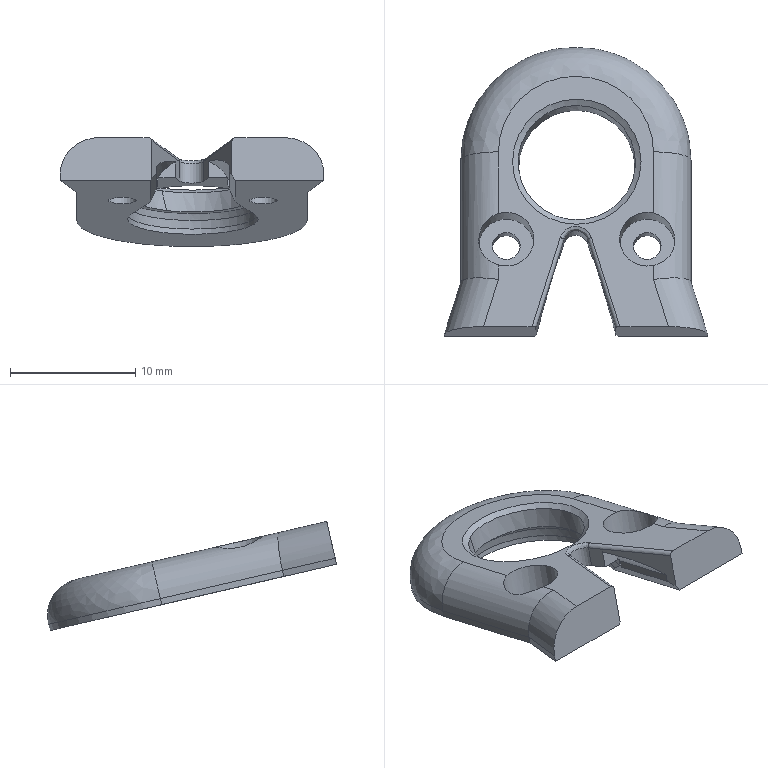Part | STEP file | 1 solid | 43 faces | box 21.033 x 23.076 x 8.696 mm | volume 790.702 mm3 | plane 21 | cylinder 14 | spline 7 | cone 1 | commonest cylinder face diameters 6 x4 0.6 x2 2.2 x2 4.4 x2 6.428 x2 2 x1